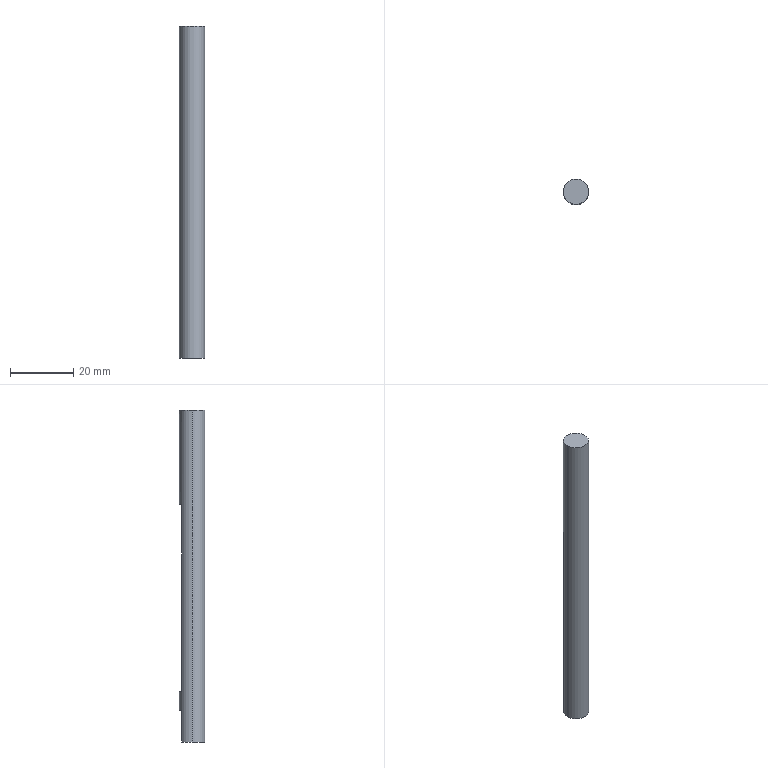Part | SolidWorks | features ICE 2, Extrusion 1 | 1 solid | 9 faces | box 8 x 8 x 105 mm | volume 5097 mm3 | plane 7 | cylinder 2 | commonest cylinder face diameters 8 x2
STEP:
#1=CARTESIAN_POINT('',(-11.896,3.2,75.));
#2=VERTEX_POINT('',#1);
#3=CARTESIAN_POINT('',(-7.096,3.2,75.));
#4=VERTEX_POINT('',#3);
#5=CARTESIAN_POINT('',(-9.496,0.,75.));
#6=DIRECTION('',(0.,0.,-1.));
#7=DIRECTION('',(-1.,0.,0.));
#8=AXIS2_PLACEMENT_3D('',#5,#6,#7);
#9=CIRCLE('',#8,4.);
#10=EDGE_CURVE('',#2,#4,#9,.T.);
#11=ORIENTED_EDGE('',*,*,#10,.F.);
#12=CARTESIAN_POINT('',(-11.896,3.2,16.));
#13=VERTEX_POINT('',#12);
#14=CARTESIAN_POINT('',(-11.896,3.2,75.));
#15=DIRECTION('',(0.,0.,-1.));
#16=VECTOR('',#15,1000.);
#17=LINE('',#14,#16);
#18=EDGE_CURVE('',#2,#13,#17,.T.);
#19=ORIENTED_EDGE('',*,*,#18,.T.);
#20=CARTESIAN_POINT('',(-7.096,3.2,16.));
#21=VERTEX_POINT('',#20);
#22=CARTESIAN_POINT('',(-9.496,0.,16.));
#23=DIRECTION('',(0.,0.,-1.));
#24=DIRECTION('',(-1.,0.,0.));
#25=AXIS2_PLACEMENT_3D('',#22,#23,#24);
#26=CIRCLE('',#25,4.);
#27=EDGE_CURVE('',#13,#21,#26,.T.);
#28=ORIENTED_EDGE('',*,*,#27,.T.);
#29=CARTESIAN_POINT('',(-7.096,3.2,75.));
#30=DIRECTION('',(0.,0.,-1.));
#31=VECTOR('',#30,1000.);
#32=LINE('',#29,#31);
#33=EDGE_CURVE('',#4,#21,#32,.T.);
#34=ORIENTED_EDGE('',*,*,#33,.F.);
#35=EDGE_LOOP('',(#11,#19,#28,#34));
#36=FACE_BOUND('',#35,.T.);
#37=CARTESIAN_POINT('',(-5.496,0.,105.));
#38=VERTEX_POINT('',#37);
#39=CARTESIAN_POINT('',(-13.496,0.,105.));
#40=VERTEX_POINT('',#39);
#41=CARTESIAN_POINT('',(-9.496,0.,105.));
#42=DIRECTION('',(0.,0.,1.));
#43=DIRECTION('',(1.,0.,0.));
#44=AXIS2_PLACEMENT_3D('',#41,#42,#43);
#45=CIRCLE('',#44,4.);
#46=EDGE_CURVE('',#38,#40,#45,.T.);
#47=ORIENTED_EDGE('',*,*,#46,.F.);
#48=CARTESIAN_POINT('',(-5.496,0.,0.));
#49=VERTEX_POINT('',#48);
#50=CARTESIAN_POINT('',(-5.496,0.,105.));
#51=DIRECTION('',(0.,0.,-1.));
#52=VECTOR('',#51,1000.);
#53=LINE('',#50,#52);
#54=EDGE_CURVE('',#38,#49,#53,.T.);
#55=ORIENTED_EDGE('',*,*,#54,.T.);
#56=CARTESIAN_POINT('',(-7.096,3.2,0.));
#57=VERTEX_POINT('',#56);
#58=CARTESIAN_POINT('',(-9.496,0.,0.));
#59=DIRECTION('',(0.,0.,1.));
#60=DIRECTION('',(1.,0.,0.));
#61=AXIS2_PLACEMENT_3D('',#58,#59,#60);
#62=CIRCLE('',#61,4.);
#63=EDGE_CURVE('',#49,#57,#62,.T.);
#64=ORIENTED_EDGE('',*,*,#63,.T.);
#65=CARTESIAN_POINT('',(-7.096,3.2,10.));
#66=VERTEX_POINT('',#65);
#67=CARTESIAN_POINT('',(-7.096,3.2,10.));
#68=DIRECTION('',(0.,0.,-1.));
#69=VECTOR('',#68,1000.);
#70=LINE('',#67,#69);
#71=EDGE_CURVE('',#66,#57,#70,.T.);
#72=ORIENTED_EDGE('',*,*,#71,.F.);
#73=CARTESIAN_POINT('',(-11.896,3.2,10.));
#74=VERTEX_POINT('',#73);
#75=CARTESIAN_POINT('',(-9.496,0.,10.));
#76=DIRECTION('',(0.,0.,-1.));
#77=DIRECTION('',(-1.,0.,0.));
#78=AXIS2_PLACEMENT_3D('',#75,#76,#77);
#79=CIRCLE('',#78,4.);
#80=EDGE_CURVE('',#74,#66,#79,.T.);
#81=ORIENTED_EDGE('',*,*,#80,.F.);
#82=CARTESIAN_POINT('',(-11.896,3.2,0.));
#83=VERTEX_POINT('',#82);
#84=CARTESIAN_POINT('',(-11.896,3.2,10.));
#85=DIRECTION('',(0.,0.,-1.));
#86=VECTOR('',#85,1000.);
#87=LINE('',#84,#86);
#88=EDGE_CURVE('',#74,#83,#87,.T.);
#89=ORIENTED_EDGE('',*,*,#88,.T.);
#90=CARTESIAN_POINT('',(-13.496,0.,0.));
#91=VERTEX_POINT('',#90);
#92=CARTESIAN_POINT('',(-9.496,0.,0.));
#93=DIRECTION('',(0.,0.,1.));
#94=DIRECTION('',(1.,0.,0.));
#95=AXIS2_PLACEMENT_3D('',#92,#93,#94);
#96=CIRCLE('',#95,4.);
#97=EDGE_CURVE('',#83,#91,#96,.T.);
#98=ORIENTED_EDGE('',*,*,#97,.T.);
#99=CARTESIAN_POINT('',(-13.496,0.,105.));
#100=DIRECTION('',(0.,0.,-1.));
#101=VECTOR('',#100,1000.);
#102=LINE('',#99,#101);
#103=EDGE_CURVE('',#40,#91,#102,.T.);
#104=ORIENTED_EDGE('',*,*,#103,.F.);
#105=EDGE_LOOP('',(#47,#55,#64,#72,#81,#89,#98,#104));
#106=FACE_OUTER_BOUND('',#105,.T.);
#107=CARTESIAN_POINT('',(-9.496,0.,105.));
#108=DIRECTION('',(0.,0.,-1.));
#109=DIRECTION('',(-1.,0.,0.));
#110=AXIS2_PLACEMENT_3D('',#107,#108,#109);
#111=CYLINDRICAL_SURFACE('',#110,4.);
#112=ADVANCED_FACE('',(#36,#106),#111,.T.);
#113=ORIENTED_EDGE('',*,*,#54,.F.);
#114=CARTESIAN_POINT('',(-9.496,0.,105.));
#115=DIRECTION('',(0.,0.,1.));
#116=DIRECTION('',(1.,0.,0.));
#117=AXIS2_PLACEMENT_3D('',#114,#115,#116);
#118=CIRCLE('',#117,4.);
#119=EDGE_CURVE('',#40,#38,#118,.T.);
#120=ORIENTED_EDGE('',*,*,#119,.F.);
#121=ORIENTED_EDGE('',*,*,#103,.T.);
#122=CARTESIAN_POINT('',(-9.496,0.,0.));
#123=DIRECTION('',(0.,0.,1.));
#124=DIRECTION('',(1.,0.,0.));
#125=AXIS2_PLACEMENT_3D('',#122,#123,#124);
#126=CIRCLE('',#125,4.);
#127=EDGE_CURVE('',#91,#49,#126,.T.);
#128=ORIENTED_EDGE('',*,*,#127,.T.);
#129=EDGE_LOOP('',(#113,#120,#121,#128));
#130=FACE_OUTER_BOUND('',#129,.T.);
#131=CARTESIAN_POINT('',(-9.496,0.,105.));
#132=DIRECTION('',(0.,0.,-1.));
#133=DIRECTION('',(-1.,0.,0.));
#134=AXIS2_PLACEMENT_3D('',#131,#132,#133);
#135=CYLINDRICAL_SURFACE('',#134,4.);
#136=ADVANCED_FACE('',(#130),#135,.T.);
#137=ORIENTED_EDGE('',*,*,#119,.T.);
#138=ORIENTED_EDGE('',*,*,#46,.T.);
#139=EDGE_LOOP('',(#137,#138));
#140=FACE_OUTER_BOUND('',#139,.T.);
#141=CARTESIAN_POINT('',(-9.496,0.,105.));
#142=DIRECTION('',(0.,0.,1.));
#143=DIRECTION('',(1.,0.,0.));
#144=AXIS2_PLACEMENT_3D('',#141,#142,#143);
#145=PLANE('',#144);
#146=ADVANCED_FACE('',(#140),#145,.T.);
#147=ORIENTED_EDGE('',*,*,#97,.F.);
#148=CARTESIAN_POINT('',(-7.096,3.2,0.));
#149=DIRECTION('',(-1.,0.,0.));
#150=VECTOR('',#149,1000.);
#151=LINE('',#148,#150);
#152=EDGE_CURVE('',#57,#83,#151,.T.);
#153=ORIENTED_EDGE('',*,*,#152,.F.);
#154=ORIENTED_EDGE('',*,*,#63,.F.);
#155=ORIENTED_EDGE('',*,*,#127,.F.);
#156=EDGE_LOOP('',(#147,#153,#154,#155));
#157=FACE_OUTER_BOUND('',#156,.T.);
#158=CARTESIAN_POINT('',(-9.496,0.,0.));
#159=DIRECTION('',(0.,0.,1.));
#160=DIRECTION('',(1.,0.,0.));
#161=AXIS2_PLACEMENT_3D('',#158,#159,#160);
#162=PLANE('',#161);
#163=ADVANCED_FACE('',(#157),#162,.F.);
#164=ORIENTED_EDGE('',*,*,#152,.T.);
#165=ORIENTED_EDGE('',*,*,#88,.F.);
#166=CARTESIAN_POINT('',(-7.096,3.2,10.));
#167=DIRECTION('',(-1.,0.,0.));
#168=VECTOR('',#167,1000.);
#169=LINE('',#166,#168);
#170=EDGE_CURVE('',#66,#74,#169,.T.);
#171=ORIENTED_EDGE('',*,*,#170,.F.);
#172=ORIENTED_EDGE('',*,*,#71,.T.);
#173=EDGE_LOOP('',(#164,#165,#171,#172));
#174=FACE_OUTER_BOUND('',#173,.T.);
#175=CARTESIAN_POINT('',(-7.096,3.2,10.));
#176=DIRECTION('',(0.,-1.,0.));
#177=DIRECTION('',(0.,0.,-1.));
#178=AXIS2_PLACEMENT_3D('',#175,#176,#177);
#179=PLANE('',#178);
#180=ADVANCED_FACE('',(#174),#179,.F.);
#181=ORIENTED_EDGE('',*,*,#80,.T.);
#182=ORIENTED_EDGE('',*,*,#170,.T.);
#183=EDGE_LOOP('',(#181,#182));
#184=FACE_OUTER_BOUND('',#183,.T.);
#185=CARTESIAN_POINT('',(-9.496,0.,10.));
#186=DIRECTION('',(0.,0.,-1.));
#187=DIRECTION('',(-1.,0.,0.));
#188=AXIS2_PLACEMENT_3D('',#185,#186,#187);
#189=PLANE('',#188);
#190=ADVANCED_FACE('',(#184),#189,.T.);
#191=CARTESIAN_POINT('',(-7.096,3.2,16.));
#192=DIRECTION('',(-1.,0.,0.));
#193=VECTOR('',#192,1000.);
#194=LINE('',#191,#193);
#195=EDGE_CURVE('',#21,#13,#194,.T.);
#196=ORIENTED_EDGE('',*,*,#195,.T.);
#197=ORIENTED_EDGE('',*,*,#18,.F.);
#198=CARTESIAN_POINT('',(-7.096,3.2,75.));
#199=DIRECTION('',(-1.,0.,0.));
#200=VECTOR('',#199,1000.);
#201=LINE('',#198,#200);
#202=EDGE_CURVE('',#4,#2,#201,.T.);
#203=ORIENTED_EDGE('',*,*,#202,.F.);
#204=ORIENTED_EDGE('',*,*,#33,.T.);
#205=EDGE_LOOP('',(#196,#197,#203,#204));
#206=FACE_OUTER_BOUND('',#205,.T.);
#207=CARTESIAN_POINT('',(-7.096,3.2,75.));
#208=DIRECTION('',(0.,-1.,0.));
#209=DIRECTION('',(0.,0.,-1.));
#210=AXIS2_PLACEMENT_3D('',#207,#208,#209);
#211=PLANE('',#210);
#212=ADVANCED_FACE('',(#206),#211,.F.);
#213=ORIENTED_EDGE('',*,*,#10,.T.);
#214=ORIENTED_EDGE('',*,*,#202,.T.);
#215=EDGE_LOOP('',(#213,#214));
#216=FACE_OUTER_BOUND('',#215,.T.);
#217=CARTESIAN_POINT('',(-9.496,0.,75.));
#218=DIRECTION('',(0.,0.,-1.));
#219=DIRECTION('',(-1.,0.,0.));
#220=AXIS2_PLACEMENT_3D('',#217,#218,#219);
#221=PLANE('',#220);
#222=ADVANCED_FACE('',(#216),#221,.T.);
#223=ORIENTED_EDGE('',*,*,#27,.F.);
#224=ORIENTED_EDGE('',*,*,#195,.F.);
#225=EDGE_LOOP('',(#223,#224));
#226=FACE_OUTER_BOUND('',#225,.T.);
#227=CARTESIAN_POINT('',(-9.496,0.,16.));
#228=DIRECTION('',(0.,0.,-1.));
#229=DIRECTION('',(-1.,0.,0.));
#230=AXIS2_PLACEMENT_3D('',#227,#228,#229);
#231=PLANE('',#230);
#232=ADVANCED_FACE('',(#226),#231,.F.);
#233=CLOSED_SHELL('',(#112,#136,#146,#163,#180,#190,#212,#222,#232));
#234=MANIFOLD_SOLID_BREP('',#233);
#235=CARTESIAN_POINT('',(0.,0.,0.));
#236=DIRECTION('',(0.,0.,1.));
#237=DIRECTION('',(1.,0.,0.));
#238=AXIS2_PLACEMENT_3D('',#235,#236,#237);
#239=(LENGTH_UNIT()NAMED_UNIT(*)SI_UNIT(.MILLI.,.METRE.));
#240=UNCERTAINTY_MEASURE_WITH_UNIT(LENGTH_MEASURE(0.00001),#239,'','');
#241=(NAMED_UNIT(*)PLANE_ANGLE_UNIT()SI_UNIT($,.RADIAN.));
#242=(NAMED_UNIT(*)SI_UNIT($,.STERADIAN.)SOLID_ANGLE_UNIT());
#243=(GEOMETRIC_REPRESENTATION_CONTEXT(3)GLOBAL_UNCERTAINTY_ASSIGNED_CONTEXT((#240))GLOBAL_UNIT_ASSIGNED_CONTEXT((#239,#241,#242))REPRESENTATION_CONTEXT('',''));
#244=ADVANCED_BREP_SHAPE_REPRESENTATION('',(#234,#238),#243);